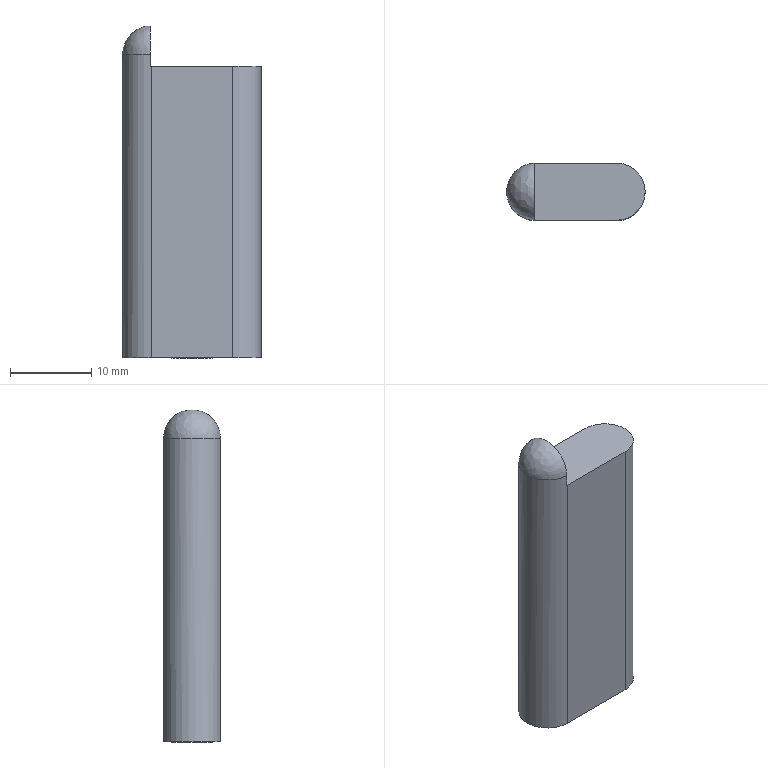Part | STEP file | LUOI GA TRON DUOI | 1 solid | 15 faces | box 17 x 7 x 40.799 mm | volume 3679 mm3 | cylinder 5 | plane 5 | cone 4 | spline 1 | commonest cylinder face diameters 7 x3 4.134 x2
STEP:
#1=CARTESIAN_POINT('',(0.,0.,0.));
#2=DIRECTION('',(0.,0.,1.));
#3=DIRECTION('',(1.,0.,0.));
#4=AXIS2_PLACEMENT_3D('',#1,#2,#3);
#5=CARTESIAN_POINT('',(-3.5,0.,0.));
#6=VERTEX_POINT('',#5);
#7=CARTESIAN_POINT('',(0.,3.5,0.));
#8=VERTEX_POINT('',#7);
#9=CARTESIAN_POINT('',(-3.5,3.5,0.));
#10=DIRECTION('',(0.,0.,1.));
#11=DIRECTION('',(1.,0.,0.));
#12=AXIS2_PLACEMENT_3D('',#9,#10,#11);
#13=CIRCLE('',#12,3.5);
#14=CARTESIAN_POINT('',(-3.5,3.5,0.));
#15=DIRECTION('',(0.,0.,1.));
#16=DIRECTION('',(1.,0.,0.));
#17=AXIS2_PLACEMENT_3D('',#14,#15,#16);
#18=CYLINDRICAL_SURFACE('',#17,3.5);
#19=CARTESIAN_POINT('',(0.,0.));
#20=DIRECTION('',(1.,0.));
#21=VECTOR('',#20,1.);
#22=LINE('',#19,#21);
#23=(GEOMETRIC_REPRESENTATION_CONTEXT(2)PARAMETRIC_REPRESENTATION_CONTEXT()REPRESENTATION_CONTEXT('',''));
#24=DEFINITIONAL_REPRESENTATION('',(#22),#23);
#25=PCURVE('',#18,#24);
#26=CARTESIAN_POINT('',(-8.5,3.5,0.));
#27=DIRECTION('',(0.,0.,1.));
#28=DIRECTION('',(1.,0.,0.));
#29=AXIS2_PLACEMENT_3D('',#26,#27,#28);
#30=PLANE('',#29);
#31=CARTESIAN_POINT('',(5.,0.));
#32=DIRECTION('',(1.,0.));
#33=AXIS2_PLACEMENT_2D('',#31,#32);
#34=CIRCLE('',#33,3.5);
#35=(GEOMETRIC_REPRESENTATION_CONTEXT(2)PARAMETRIC_REPRESENTATION_CONTEXT()REPRESENTATION_CONTEXT('',''));
#36=DEFINITIONAL_REPRESENTATION('',(#34),#35);
#37=PCURVE('',#30,#36);
#38=SURFACE_CURVE('',#13,(#25,#37),.PCURVE_S1.);
#39=EDGE_CURVE('',#6,#8,#38,.T.);
#40=ORIENTED_EDGE('',*,*,#39,.T.);
#41=CARTESIAN_POINT('',(0.,3.5,35.8));
#42=VERTEX_POINT('',#41);
#43=CARTESIAN_POINT('',(0.,3.5,0.));
#44=DIRECTION('',(0.,0.,1.));
#45=VECTOR('',#44,1.);
#46=LINE('',#43,#45);
#47=CARTESIAN_POINT('',(6.283,0.));
#48=DIRECTION('',(0.,1.));
#49=VECTOR('',#48,1.);
#50=LINE('',#47,#49);
#51=(GEOMETRIC_REPRESENTATION_CONTEXT(2)PARAMETRIC_REPRESENTATION_CONTEXT()REPRESENTATION_CONTEXT('',''));
#52=DEFINITIONAL_REPRESENTATION('',(#50),#51);
#53=PCURVE('',#18,#52);
#54=CARTESIAN_POINT('',(-3.5,3.5,0.));
#55=DIRECTION('',(0.,0.,1.));
#56=DIRECTION('',(1.,0.,0.));
#57=AXIS2_PLACEMENT_3D('',#54,#55,#56);
#58=CYLINDRICAL_SURFACE('',#57,3.5);
#59=CARTESIAN_POINT('',(0.,0.));
#60=DIRECTION('',(0.,1.));
#61=VECTOR('',#60,1.);
#62=LINE('',#59,#61);
#63=(GEOMETRIC_REPRESENTATION_CONTEXT(2)PARAMETRIC_REPRESENTATION_CONTEXT()REPRESENTATION_CONTEXT('',''));
#64=DEFINITIONAL_REPRESENTATION('',(#62),#63);
#65=PCURVE('',#58,#64);
#66=SURFACE_CURVE('',#46,(#53,#65),.PCURVE_S1.);
#67=EDGE_CURVE('',#8,#42,#66,.T.);
#68=ORIENTED_EDGE('',*,*,#67,.T.);
#69=CARTESIAN_POINT('',(-3.5,0.,35.8));
#70=VERTEX_POINT('',#69);
#71=CARTESIAN_POINT('',(-3.5,3.5,35.8));
#72=DIRECTION('',(0.,0.,-1.));
#73=DIRECTION('',(1.,0.,0.));
#74=AXIS2_PLACEMENT_3D('',#71,#72,#73);
#75=CIRCLE('',#74,3.5);
#76=CARTESIAN_POINT('',(6.283,35.8));
#77=DIRECTION('',(-1.,0.));
#78=VECTOR('',#77,1.);
#79=LINE('',#76,#78);
#80=(GEOMETRIC_REPRESENTATION_CONTEXT(2)PARAMETRIC_REPRESENTATION_CONTEXT()REPRESENTATION_CONTEXT('',''));
#81=DEFINITIONAL_REPRESENTATION('',(#79),#80);
#82=PCURVE('',#18,#81);
#83=CARTESIAN_POINT('',(-13.6,0.,35.8));
#84=DIRECTION('',(0.,0.,-1.));
#85=DIRECTION('',(-1.,0.,0.));
#86=AXIS2_PLACEMENT_3D('',#83,#84,#85);
#87=PLANE('',#86);
#88=CARTESIAN_POINT('',(-10.1,3.5));
#89=DIRECTION('',(-1.,0.));
#90=AXIS2_PLACEMENT_2D('',#88,#89);
#91=CIRCLE('',#90,3.5);
#92=(GEOMETRIC_REPRESENTATION_CONTEXT(2)PARAMETRIC_REPRESENTATION_CONTEXT()REPRESENTATION_CONTEXT('',''));
#93=DEFINITIONAL_REPRESENTATION('',(#91),#92);
#94=PCURVE('',#87,#93);
#95=SURFACE_CURVE('',#75,(#82,#94),.PCURVE_S1.);
#96=EDGE_CURVE('',#42,#70,#95,.T.);
#97=ORIENTED_EDGE('',*,*,#96,.T.);
#98=CARTESIAN_POINT('',(-3.5,0.,0.));
#99=DIRECTION('',(0.,0.,1.));
#100=VECTOR('',#99,1.);
#101=LINE('',#98,#100);
#102=CARTESIAN_POINT('',(4.712,0.));
#103=DIRECTION('',(0.,1.));
#104=VECTOR('',#103,1.);
#105=LINE('',#102,#104);
#106=(GEOMETRIC_REPRESENTATION_CONTEXT(2)PARAMETRIC_REPRESENTATION_CONTEXT()REPRESENTATION_CONTEXT('',''));
#107=DEFINITIONAL_REPRESENTATION('',(#105),#106);
#108=PCURVE('',#18,#107);
#109=CARTESIAN_POINT('',(0.,0.,0.));
#110=DIRECTION('',(0.,-1.,0.));
#111=DIRECTION('',(0.,0.,-1.));
#112=AXIS2_PLACEMENT_3D('',#109,#110,#111);
#113=PLANE('',#112);
#114=CARTESIAN_POINT('',(0.,-3.5));
#115=DIRECTION('',(-1.,0.));
#116=VECTOR('',#115,1.);
#117=LINE('',#114,#116);
#118=(GEOMETRIC_REPRESENTATION_CONTEXT(2)PARAMETRIC_REPRESENTATION_CONTEXT()REPRESENTATION_CONTEXT('',''));
#119=DEFINITIONAL_REPRESENTATION('',(#117),#118);
#120=PCURVE('',#113,#119);
#121=SURFACE_CURVE('',#101,(#108,#120),.PCURVE_S1.);
#122=EDGE_CURVE('',#6,#70,#121,.T.);
#123=ORIENTED_EDGE('',*,*,#122,.F.);
#124=EDGE_LOOP('',(#40,#68,#97,#123));
#125=FACE_BOUND('',#124,.T.);
#126=ADVANCED_FACE('',(#125),#18,.T.);
#127=CARTESIAN_POINT('',(-10.567,3.5,0.5));
#128=VERTEX_POINT('',#127);
#129=CARTESIAN_POINT('',(-11.067,3.5,0.));
#130=VERTEX_POINT('',#129);
#131=CARTESIAN_POINT('',(-11.067,3.5,0.));
#132=DIRECTION('',(-0.7071,0.,-0.7071));
#133=VECTOR('',#132,1.);
#134=LINE('',#131,#133);
#135=CARTESIAN_POINT('',(-8.5,3.5,0.));
#136=DIRECTION('',(0.,0.,-1.));
#137=DIRECTION('',(-1.,0.,0.));
#138=AXIS2_PLACEMENT_3D('',#135,#136,#137);
#139=CONICAL_SURFACE('',#138,2.567,0.7854);
#140=CARTESIAN_POINT('',(6.283,0.));
#141=DIRECTION('',(0.,1.));
#142=VECTOR('',#141,1.);
#143=LINE('',#140,#142);
#144=(GEOMETRIC_REPRESENTATION_CONTEXT(2)PARAMETRIC_REPRESENTATION_CONTEXT()REPRESENTATION_CONTEXT('',''));
#145=DEFINITIONAL_REPRESENTATION('',(#143),#144);
#146=PCURVE('',#139,#145);
#147=CARTESIAN_POINT('',(-8.5,3.5,0.));
#148=DIRECTION('',(0.,0.,-1.));
#149=DIRECTION('',(-1.,0.,0.));
#150=AXIS2_PLACEMENT_3D('',#147,#148,#149);
#151=CONICAL_SURFACE('',#150,2.567,0.7854);
#152=CARTESIAN_POINT('',(0.,0.));
#153=DIRECTION('',(0.,1.));
#154=VECTOR('',#153,1.);
#155=LINE('',#152,#154);
#156=(GEOMETRIC_REPRESENTATION_CONTEXT(2)PARAMETRIC_REPRESENTATION_CONTEXT()REPRESENTATION_CONTEXT('',''));
#157=DEFINITIONAL_REPRESENTATION('',(#155),#156);
#158=PCURVE('',#151,#157);
#159=SURFACE_CURVE('',#134,(#146,#158),.PCURVE_S1.);
#160=EDGE_CURVE('',#128,#130,#159,.T.);
#161=ORIENTED_EDGE('',*,*,#160,.T.);
#162=CARTESIAN_POINT('',(-5.933,3.5,0.));
#163=VERTEX_POINT('',#162);
#164=CARTESIAN_POINT('',(-8.5,3.5,0.));
#165=DIRECTION('',(0.,0.,-1.));
#166=DIRECTION('',(-1.,0.,0.));
#167=AXIS2_PLACEMENT_3D('',#164,#165,#166);
#168=CIRCLE('',#167,2.567);
#169=CARTESIAN_POINT('',(0.,0.));
#170=DIRECTION('',(1.,0.));
#171=VECTOR('',#170,1.);
#172=LINE('',#169,#171);
#173=(GEOMETRIC_REPRESENTATION_CONTEXT(2)PARAMETRIC_REPRESENTATION_CONTEXT()REPRESENTATION_CONTEXT('',''));
#174=DEFINITIONAL_REPRESENTATION('',(#172),#173);
#175=PCURVE('',#139,#174);
#176=CARTESIAN_POINT('',(-2.567,0.));
#177=CARTESIAN_POINT('',(-2.567,4.446));
#178=CARTESIAN_POINT('',(1.283,2.223));
#179=CARTESIAN_POINT('',(5.134,0.));
#180=CARTESIAN_POINT('',(1.283,-2.223));
#181=CARTESIAN_POINT('',(-2.567,-4.446));
#182=CARTESIAN_POINT('',(-2.567,0.));
#183=(BOUNDED_CURVE()B_SPLINE_CURVE(2,(#176,#177,#178,#179,#180,#181,#182),.UNSPECIFIED.,.T.,.F.)B_SPLINE_CURVE_WITH_KNOTS((1,2,2,2,2,1),(-2.094,0.,2.094,4.189,6.283,8.378),.UNSPECIFIED.)CURVE()GEOMETRIC_REPRESENTATION_ITEM()RATIONAL_B_SPLINE_CURVE((1.,0.5,1.,0.5,1.,0.5,1.))REPRESENTATION_ITEM(''));
#184=(GEOMETRIC_REPRESENTATION_CONTEXT(2)PARAMETRIC_REPRESENTATION_CONTEXT()REPRESENTATION_CONTEXT('',''));
#185=DEFINITIONAL_REPRESENTATION('',(#183),#184);
#186=PCURVE('',#30,#185);
#187=SURFACE_CURVE('',#168,(#175,#186),.PCURVE_S1.);
#188=EDGE_CURVE('',#163,#130,#187,.T.);
#189=ORIENTED_EDGE('',*,*,#188,.F.);
#190=CARTESIAN_POINT('',(-6.433,3.5,0.5));
#191=VERTEX_POINT('',#190);
#192=CARTESIAN_POINT('',(-5.933,3.5,0.));
#193=DIRECTION('',(0.7071,0.,-0.7071));
#194=VECTOR('',#193,1.);
#195=LINE('',#192,#194);
#196=CARTESIAN_POINT('',(3.142,0.));
#197=DIRECTION('',(0.,1.));
#198=VECTOR('',#197,1.);
#199=LINE('',#196,#198);
#200=(GEOMETRIC_REPRESENTATION_CONTEXT(2)PARAMETRIC_REPRESENTATION_CONTEXT()REPRESENTATION_CONTEXT('',''));
#201=DEFINITIONAL_REPRESENTATION('',(#199),#200);
#202=PCURVE('',#139,#201);
#203=CARTESIAN_POINT('',(3.142,0.));
#204=DIRECTION('',(0.,1.));
#205=VECTOR('',#204,1.);
#206=LINE('',#203,#205);
#207=(GEOMETRIC_REPRESENTATION_CONTEXT(2)PARAMETRIC_REPRESENTATION_CONTEXT()REPRESENTATION_CONTEXT('',''));
#208=DEFINITIONAL_REPRESENTATION('',(#206),#207);
#209=PCURVE('',#151,#208);
#210=SURFACE_CURVE('',#195,(#202,#209),.PCURVE_S1.);
#211=EDGE_CURVE('',#191,#163,#210,.T.);
#212=ORIENTED_EDGE('',*,*,#211,.F.);
#213=CARTESIAN_POINT('',(-8.5,3.5,0.5));
#214=DIRECTION('',(0.,0.,-1.));
#215=DIRECTION('',(1.,0.,0.));
#216=AXIS2_PLACEMENT_3D('',#213,#214,#215);
#217=CIRCLE('',#216,2.067);
#218=CARTESIAN_POINT('',(3.142,-0.5));
#219=DIRECTION('',(1.,0.));
#220=VECTOR('',#219,1.);
#221=LINE('',#218,#220);
#222=(GEOMETRIC_REPRESENTATION_CONTEXT(2)PARAMETRIC_REPRESENTATION_CONTEXT()REPRESENTATION_CONTEXT('',''));
#223=DEFINITIONAL_REPRESENTATION('',(#221),#222);
#224=PCURVE('',#139,#223);
#225=CARTESIAN_POINT('',(-8.5,3.5,10.));
#226=DIRECTION('',(0.,0.,-1.));
#227=DIRECTION('',(-1.,0.,0.));
#228=AXIS2_PLACEMENT_3D('',#225,#226,#227);
#229=CYLINDRICAL_SURFACE('',#228,2.067);
#230=CARTESIAN_POINT('',(3.142,9.5));
#231=DIRECTION('',(1.,0.));
#232=VECTOR('',#231,1.);
#233=LINE('',#230,#232);
#234=(GEOMETRIC_REPRESENTATION_CONTEXT(2)PARAMETRIC_REPRESENTATION_CONTEXT()REPRESENTATION_CONTEXT('',''));
#235=DEFINITIONAL_REPRESENTATION('',(#233),#234);
#236=PCURVE('',#229,#235);
#237=SURFACE_CURVE('',#217,(#224,#236),.PCURVE_S1.);
#238=EDGE_CURVE('',#191,#128,#237,.T.);
#239=ORIENTED_EDGE('',*,*,#238,.T.);
#240=EDGE_LOOP('',(#161,#189,#212,#239));
#241=FACE_BOUND('',#240,.F.);
#242=ADVANCED_FACE('',(#241),#139,.F.);
#243=CARTESIAN_POINT('',(-10.567,3.5,20.));
#244=VERTEX_POINT('',#243);
#245=CARTESIAN_POINT('',(-10.567,3.5,10.));
#246=DIRECTION('',(0.,0.,-1.));
#247=VECTOR('',#246,1.);
#248=LINE('',#245,#247);
#249=CARTESIAN_POINT('',(6.283,0.));
#250=DIRECTION('',(0.,1.));
#251=VECTOR('',#250,1.);
#252=LINE('',#249,#251);
#253=(GEOMETRIC_REPRESENTATION_CONTEXT(2)PARAMETRIC_REPRESENTATION_CONTEXT()REPRESENTATION_CONTEXT('',''));
#254=DEFINITIONAL_REPRESENTATION('',(#252),#253);
#255=PCURVE('',#229,#254);
#256=CARTESIAN_POINT('',(-8.5,3.5,10.));
#257=DIRECTION('',(0.,0.,-1.));
#258=DIRECTION('',(-1.,0.,0.));
#259=AXIS2_PLACEMENT_3D('',#256,#257,#258);
#260=CYLINDRICAL_SURFACE('',#259,2.067);
#261=CARTESIAN_POINT('',(0.,0.));
#262=DIRECTION('',(0.,1.));
#263=VECTOR('',#262,1.);
#264=LINE('',#261,#263);
#265=(GEOMETRIC_REPRESENTATION_CONTEXT(2)PARAMETRIC_REPRESENTATION_CONTEXT()REPRESENTATION_CONTEXT('',''));
#266=DEFINITIONAL_REPRESENTATION('',(#264),#265);
#267=PCURVE('',#260,#266);
#268=SURFACE_CURVE('',#248,(#255,#267),.PCURVE_S1.);
#269=EDGE_CURVE('',#244,#128,#268,.T.);
#270=ORIENTED_EDGE('',*,*,#269,.T.);
#271=ORIENTED_EDGE('',*,*,#238,.F.);
#272=CARTESIAN_POINT('',(-6.433,3.5,20.));
#273=VERTEX_POINT('',#272);
#274=CARTESIAN_POINT('',(-6.433,3.5,10.));
#275=DIRECTION('',(0.,0.,-1.));
#276=VECTOR('',#275,1.);
#277=LINE('',#274,#276);
#278=CARTESIAN_POINT('',(3.142,0.));
#279=DIRECTION('',(0.,1.));
#280=VECTOR('',#279,1.);
#281=LINE('',#278,#280);
#282=(GEOMETRIC_REPRESENTATION_CONTEXT(2)PARAMETRIC_REPRESENTATION_CONTEXT()REPRESENTATION_CONTEXT('',''));
#283=DEFINITIONAL_REPRESENTATION('',(#281),#282);
#284=PCURVE('',#229,#283);
#285=CARTESIAN_POINT('',(3.142,0.));
#286=DIRECTION('',(0.,1.));
#287=VECTOR('',#286,1.);
#288=LINE('',#285,#287);
#289=(GEOMETRIC_REPRESENTATION_CONTEXT(2)PARAMETRIC_REPRESENTATION_CONTEXT()REPRESENTATION_CONTEXT('',''));
#290=DEFINITIONAL_REPRESENTATION('',(#288),#289);
#291=PCURVE('',#260,#290);
#292=SURFACE_CURVE('',#277,(#284,#291),.PCURVE_S1.);
#293=EDGE_CURVE('',#273,#191,#292,.T.);
#294=ORIENTED_EDGE('',*,*,#293,.F.);
#295=CARTESIAN_POINT('',(-8.5,3.5,20.));
#296=DIRECTION('',(0.,0.,-1.));
#297=DIRECTION('',(-1.,0.,0.));
#298=AXIS2_PLACEMENT_3D('',#295,#296,#297);
#299=CIRCLE('',#298,2.067);
#300=CARTESIAN_POINT('',(0.,-10.));
#301=DIRECTION('',(1.,0.));
#302=VECTOR('',#301,1.);
#303=LINE('',#300,#302);
#304=(GEOMETRIC_REPRESENTATION_CONTEXT(2)PARAMETRIC_REPRESENTATION_CONTEXT()REPRESENTATION_CONTEXT('',''));
#305=DEFINITIONAL_REPRESENTATION('',(#303),#304);
#306=PCURVE('',#229,#305);
#307=CARTESIAN_POINT('',(-8.5,3.5,20.));
#308=DIRECTION('',(0.,0.,-1.));
#309=DIRECTION('',(-1.,0.,0.));
#310=AXIS2_PLACEMENT_3D('',#307,#308,#309);
#311=CONICAL_SURFACE('',#310,2.067,1.03);
#312=CARTESIAN_POINT('',(0.,0.));
#313=DIRECTION('',(1.,0.));
#314=VECTOR('',#313,1.);
#315=LINE('',#312,#314);
#316=(GEOMETRIC_REPRESENTATION_CONTEXT(2)PARAMETRIC_REPRESENTATION_CONTEXT()REPRESENTATION_CONTEXT('',''));
#317=DEFINITIONAL_REPRESENTATION('',(#315),#316);
#318=PCURVE('',#311,#317);
#319=SURFACE_CURVE('',#299,(#306,#318),.PCURVE_S1.);
#320=EDGE_CURVE('',#273,#244,#319,.T.);
#321=ORIENTED_EDGE('',*,*,#320,.T.);
#322=EDGE_LOOP('',(#270,#271,#294,#321));
#323=FACE_BOUND('',#322,.F.);
#324=ADVANCED_FACE('',(#323),#229,.F.);
#325=ORIENTED_EDGE('',*,*,#320,.F.);
#326=CARTESIAN_POINT('',(-8.5,3.5,21.242));
#327=VERTEX_POINT('',#326);
#328=CARTESIAN_POINT('',(-6.433,3.5,20.));
#329=DIRECTION('',(0.8572,0.,-0.515));
#330=VECTOR('',#329,1.);
#331=LINE('',#328,#330);
#332=CARTESIAN_POINT('',(3.142,0.));
#333=DIRECTION('',(0.,1.));
#334=VECTOR('',#333,1.);
#335=LINE('',#332,#334);
#336=(GEOMETRIC_REPRESENTATION_CONTEXT(2)PARAMETRIC_REPRESENTATION_CONTEXT()REPRESENTATION_CONTEXT('',''));
#337=DEFINITIONAL_REPRESENTATION('',(#335),#336);
#338=PCURVE('',#311,#337);
#339=CARTESIAN_POINT('',(-8.5,3.5,20.));
#340=DIRECTION('',(0.,0.,-1.));
#341=DIRECTION('',(-1.,0.,0.));
#342=AXIS2_PLACEMENT_3D('',#339,#340,#341);
#343=CONICAL_SURFACE('',#342,2.067,1.03);
#344=CARTESIAN_POINT('',(3.142,0.));
#345=DIRECTION('',(0.,1.));
#346=VECTOR('',#345,1.);
#347=LINE('',#344,#346);
#348=(GEOMETRIC_REPRESENTATION_CONTEXT(2)PARAMETRIC_REPRESENTATION_CONTEXT()REPRESENTATION_CONTEXT('',''));
#349=DEFINITIONAL_REPRESENTATION('',(#347),#348);
#350=PCURVE('',#343,#349);
#351=SURFACE_CURVE('',#331,(#338,#350),.PCURVE_S1.);
#352=EDGE_CURVE('',#327,#273,#351,.T.);
#353=ORIENTED_EDGE('',*,*,#352,.F.);
#354=CARTESIAN_POINT('',(-10.567,3.5,20.));
#355=DIRECTION('',(-0.8572,0.,-0.515));
#356=VECTOR('',#355,1.);
#357=LINE('',#354,#356);
#358=CARTESIAN_POINT('',(6.283,0.));
#359=DIRECTION('',(0.,1.));
#360=VECTOR('',#359,1.);
#361=LINE('',#358,#360);
#362=(GEOMETRIC_REPRESENTATION_CONTEXT(2)PARAMETRIC_REPRESENTATION_CONTEXT()REPRESENTATION_CONTEXT('',''));
#363=DEFINITIONAL_REPRESENTATION('',(#361),#362);
#364=PCURVE('',#311,#363);
#365=CARTESIAN_POINT('',(0.,0.));
#366=DIRECTION('',(0.,1.));
#367=VECTOR('',#366,1.);
#368=LINE('',#365,#367);
#369=(GEOMETRIC_REPRESENTATION_CONTEXT(2)PARAMETRIC_REPRESENTATION_CONTEXT()REPRESENTATION_CONTEXT('',''));
#370=DEFINITIONAL_REPRESENTATION('',(#368),#369);
#371=PCURVE('',#343,#370);
#372=SURFACE_CURVE('',#357,(#364,#371),.PCURVE_S1.);
#373=EDGE_CURVE('',#327,#244,#372,.T.);
#374=ORIENTED_EDGE('',*,*,#373,.T.);
#375=EDGE_LOOP('',(#325,#353,#374));
#376=FACE_BOUND('',#375,.F.);
#377=ADVANCED_FACE('',(#376),#311,.F.);
#378=CARTESIAN_POINT('',(-13.5,0.,35.8));
#379=VERTEX_POINT('',#378);
#380=CARTESIAN_POINT('',(-13.6,0.001429,35.8));
#381=VERTEX_POINT('',#380);
#382=CARTESIAN_POINT('',(-13.5,3.5,35.8));
#383=DIRECTION('',(0.,0.,-1.));
#384=DIRECTION('',(1.,0.,0.));
#385=AXIS2_PLACEMENT_3D('',#382,#383,#384);
#386=CIRCLE('',#385,3.5);
#387=CARTESIAN_POINT('',(-13.5,3.5,0.));
#388=DIRECTION('',(0.,0.,1.));
#389=DIRECTION('',(1.,0.,0.));
#390=AXIS2_PLACEMENT_3D('',#387,#388,#389);
#391=CYLINDRICAL_SURFACE('',#390,3.5);
#392=CARTESIAN_POINT('',(6.283,35.8));
#393=DIRECTION('',(-1.,0.));
#394=VECTOR('',#393,1.);
#395=LINE('',#392,#394);
#396=(GEOMETRIC_REPRESENTATION_CONTEXT(2)PARAMETRIC_REPRESENTATION_CONTEXT()REPRESENTATION_CONTEXT('',''));
#397=DEFINITIONAL_REPRESENTATION('',(#395),#396);
#398=PCURVE('',#391,#397);
#399=CARTESIAN_POINT('',(-0.1,3.5));
#400=DIRECTION('',(-1.,0.));
#401=AXIS2_PLACEMENT_2D('',#399,#400);
#402=CIRCLE('',#401,3.5);
#403=(GEOMETRIC_REPRESENTATION_CONTEXT(2)PARAMETRIC_REPRESENTATION_CONTEXT()REPRESENTATION_CONTEXT('',''));
#404=DEFINITIONAL_REPRESENTATION('',(#402),#403);
#405=PCURVE('',#87,#404);
#406=SURFACE_CURVE('',#386,(#398,#405),.PCURVE_S1.);
#407=EDGE_CURVE('',#379,#381,#406,.T.);
#408=ORIENTED_EDGE('',*,*,#407,.T.);
#409=CARTESIAN_POINT('',(-13.6,0.001429,37.3));
#410=VERTEX_POINT('',#409);
#411=CARTESIAN_POINT('',(-13.6,0.001429,40.8));
#412=DIRECTION('',(0.,0.,1.));
#413=VECTOR('',#412,1.);
#414=LINE('',#411,#413);
#415=CARTESIAN_POINT('',(4.684,40.8));
#416=DIRECTION('',(0.,1.));
#417=VECTOR('',#416,1.);
#418=LINE('',#415,#417);
#419=(GEOMETRIC_REPRESENTATION_CONTEXT(2)PARAMETRIC_REPRESENTATION_CONTEXT()REPRESENTATION_CONTEXT('',''));
#420=DEFINITIONAL_REPRESENTATION('',(#418),#419);
#421=PCURVE('',#391,#420);
#422=CARTESIAN_POINT('',(-13.6,0.,40.8));
#423=DIRECTION('',(-1.,0.,0.));
#424=DIRECTION('',(0.,0.,1.));
#425=AXIS2_PLACEMENT_3D('',#422,#423,#424);
#426=PLANE('',#425);
#427=CARTESIAN_POINT('',(0.,0.001429));
#428=DIRECTION('',(1.,0.));
#429=VECTOR('',#428,1.);
#430=LINE('',#427,#429);
#431=(GEOMETRIC_REPRESENTATION_CONTEXT(2)PARAMETRIC_REPRESENTATION_CONTEXT()REPRESENTATION_CONTEXT('',''));
#432=DEFINITIONAL_REPRESENTATION('',(#430),#431);
#433=PCURVE('',#426,#432);
#434=SURFACE_CURVE('',#414,(#421,#433),.PCURVE_S1.);
#435=EDGE_CURVE('',#381,#410,#434,.T.);
#436=ORIENTED_EDGE('',*,*,#435,.T.);
#437=CARTESIAN_POINT('',(-17.,3.5,37.3));
#438=VERTEX_POINT('',#437);
#439=CARTESIAN_POINT('',(-13.5,3.5,37.3));
#440=DIRECTION('',(0.,0.,-1.));
#441=DIRECTION('',(1.,0.,0.));
#442=AXIS2_PLACEMENT_3D('',#439,#440,#441);
#443=CIRCLE('',#442,3.5);
#444=CARTESIAN_POINT('',(6.283,37.3));
#445=DIRECTION('',(-1.,0.));
#446=VECTOR('',#445,1.);
#447=LINE('',#444,#446);
#448=(GEOMETRIC_REPRESENTATION_CONTEXT(2)PARAMETRIC_REPRESENTATION_CONTEXT()REPRESENTATION_CONTEXT('',''));
#449=DEFINITIONAL_REPRESENTATION('',(#447),#448);
#450=PCURVE('',#391,#449);
#451=CARTESIAN_POINT('',(-13.6,6.999,37.3));
#452=CARTESIAN_POINT('',(-13.6,6.999,44.297));
#453=CARTESIAN_POINT('',(-13.6,0.001429,44.297));
#454=CARTESIAN_POINT('',(-13.6,0.001429,37.3));
#455=CARTESIAN_POINT('',(-15.603,6.941,37.3));
#456=CARTESIAN_POINT('',(-15.603,6.941,44.183));
#457=CARTESIAN_POINT('',(-15.603,0.05869,44.183));
#458=CARTESIAN_POINT('',(-15.603,0.05869,37.3));
#459=CARTESIAN_POINT('',(-17.,5.504,37.3));
#460=CARTESIAN_POINT('',(-17.,5.504,41.308));
#461=CARTESIAN_POINT('',(-17.,1.496,41.308));
#462=CARTESIAN_POINT('',(-17.,1.496,37.3));
#463=CARTESIAN_POINT('',(-17.,3.5,37.3));
#464=CARTESIAN_POINT('',(-17.,3.5,37.3));
#465=CARTESIAN_POINT('',(-17.,3.5,37.3));
#466=CARTESIAN_POINT('',(-17.,3.5,37.3));
#467=(BOUNDED_SURFACE()B_SPLINE_SURFACE(3,3,((#451,#452,#453,#454),(#455,#456,#457,#458),(#459,#460,#461,#462),(#463,#464,#465,#466)),.UNSPECIFIED.,.F.,.F.,.F.)B_SPLINE_SURFACE_WITH_KNOTS((4,4),(4,4),(0.,1.),(0.,1.),.PIECEWISE_BEZIER_KNOTS.)GEOMETRIC_REPRESENTATION_ITEM()RATIONAL_B_SPLINE_SURFACE(((1.,0.3333,0.3333,1.),(0.8114,0.2705,0.2705,0.8114),(0.8114,0.2705,0.2705,0.8114),(1.,0.3333,0.3333,1.)))REPRESENTATION_ITEM('')SURFACE());
#468=CARTESIAN_POINT('',(0.,1.));
#469=CARTESIAN_POINT('',(0.01676,1.));
#470=CARTESIAN_POINT('',(0.04982,1.));
#471=CARTESIAN_POINT('',(0.09814,1.));
#472=CARTESIAN_POINT('',(0.1454,1.));
#473=CARTESIAN_POINT('',(0.1917,1.));
#474=CARTESIAN_POINT('',(0.2371,1.));
#475=CARTESIAN_POINT('',(0.282,1.));
#476=CARTESIAN_POINT('',(0.3262,1.));
#477=CARTESIAN_POINT('',(0.37,1.));
#478=CARTESIAN_POINT('',(0.4135,1.));
#479=CARTESIAN_POINT('',(0.4568,1.));
#480=CARTESIAN_POINT('',(0.5,1.));
#481=CARTESIAN_POINT('',(0.5432,1.));
#482=CARTESIAN_POINT('',(0.5865,1.));
#483=CARTESIAN_POINT('',(0.63,1.));
#484=CARTESIAN_POINT('',(0.6738,1.));
#485=CARTESIAN_POINT('',(0.718,1.));
#486=CARTESIAN_POINT('',(0.7629,1.));
#487=CARTESIAN_POINT('',(0.8083,1.));
#488=CARTESIAN_POINT('',(0.8546,1.));
#489=CARTESIAN_POINT('',(0.9019,1.));
#490=CARTESIAN_POINT('',(0.9502,1.));
#491=CARTESIAN_POINT('',(0.9832,1.));
#492=CARTESIAN_POINT('',(1.,1.));
#493=B_SPLINE_CURVE_WITH_KNOTS('',3,(#468,#469,#470,#471,#472,#473,#474,#475,#476,#477,#478,#479,#480,#481,#482,#483,#484,#485,#486,#487,#488,#489,#490,#491,#492),.UNSPECIFIED.,.F.,.F.,(4,1,1,1,1,1,1,1,1,1,1,1,1,1,1,1,1,1,1,1,1,1,4),(1.599,1.669,1.74,1.81,1.88,1.95,2.02,2.09,2.16,2.23,2.3,2.37,2.441,2.511,2.581,2.651,2.721,2.791,2.861,2.931,3.001,3.071,3.142),.QUASI_UNIFORM_KNOTS.);
#494=(GEOMETRIC_REPRESENTATION_CONTEXT(2)PARAMETRIC_REPRESENTATION_CONTEXT()REPRESENTATION_CONTEXT('',''));
#495=DEFINITIONAL_REPRESENTATION('',(#493),#494);
#496=PCURVE('',#467,#495);
#497=SURFACE_CURVE('',#443,(#450,#496),.PCURVE_S1.);
#498=EDGE_CURVE('',#410,#438,#497,.T.);
#499=ORIENTED_EDGE('',*,*,#498,.T.);
#500=CARTESIAN_POINT('',(-13.6,6.999,37.3));
#501=VERTEX_POINT('',#500);
#502=CARTESIAN_POINT('',(-13.5,3.5,37.3));
#503=DIRECTION('',(0.,0.,-1.));
#504=DIRECTION('',(1.,0.,0.));
#505=AXIS2_PLACEMENT_3D('',#502,#503,#504);
#506=CIRCLE('',#505,3.5);
#507=CARTESIAN_POINT('',(6.283,37.3));
#508=DIRECTION('',(-1.,0.));
#509=VECTOR('',#508,1.);
#510=LINE('',#507,#509);
#511=(GEOMETRIC_REPRESENTATION_CONTEXT(2)PARAMETRIC_REPRESENTATION_CONTEXT()REPRESENTATION_CONTEXT('',''));
#512=DEFINITIONAL_REPRESENTATION('',(#510),#511);
#513=PCURVE('',#391,#512);
#514=CARTESIAN_POINT('',(1.,0.));
#515=CARTESIAN_POINT('',(0.9832,0.));
#516=CARTESIAN_POINT('',(0.9502,0.));
#517=CARTESIAN_POINT('',(0.9019,0.));
#518=CARTESIAN_POINT('',(0.8546,0.));
#519=CARTESIAN_POINT('',(0.8083,0.));
#520=CARTESIAN_POINT('',(0.7629,0.));
#521=CARTESIAN_POINT('',(0.718,0.));
#522=CARTESIAN_POINT('',(0.6738,0.));
#523=CARTESIAN_POINT('',(0.63,0.));
#524=CARTESIAN_POINT('',(0.5865,0.));
#525=CARTESIAN_POINT('',(0.5432,0.));
#526=CARTESIAN_POINT('',(0.5,0.));
#527=CARTESIAN_POINT('',(0.4568,0.));
#528=CARTESIAN_POINT('',(0.4135,0.));
#529=CARTESIAN_POINT('',(0.37,0.));
#530=CARTESIAN_POINT('',(0.3262,0.));
#531=CARTESIAN_POINT('',(0.282,0.));
#532=CARTESIAN_POINT('',(0.2371,0.));
#533=CARTESIAN_POINT('',(0.1917,0.));
#534=CARTESIAN_POINT('',(0.1454,0.));
#535=CARTESIAN_POINT('',(0.09814,0.));
#536=CARTESIAN_POINT('',(0.04982,0.));
#537=CARTESIAN_POINT('',(0.01676,0.));
#538=CARTESIAN_POINT('',(0.,0.));
#539=B_SPLINE_CURVE_WITH_KNOTS('',3,(#514,#515,#516,#517,#518,#519,#520,#521,#522,#523,#524,#525,#526,#527,#528,#529,#530,#531,#532,#533,#534,#535,#536,#537,#538),.UNSPECIFIED.,.F.,.F.,(4,1,1,1,1,1,1,1,1,1,1,1,1,1,1,1,1,1,1,1,1,1,4),(3.142,3.212,3.282,3.352,3.422,3.492,3.562,3.632,3.702,3.773,3.843,3.913,3.983,4.053,4.123,4.193,4.263,4.333,4.403,4.474,4.544,4.614,4.684),.QUASI_UNIFORM_KNOTS.);
#540=(GEOMETRIC_REPRESENTATION_CONTEXT(2)PARAMETRIC_REPRESENTATION_CONTEXT()REPRESENTATION_CONTEXT('',''));
#541=DEFINITIONAL_REPRESENTATION('',(#539),#540);
#542=PCURVE('',#467,#541);
#543=SURFACE_CURVE('',#506,(#513,#542),.PCURVE_S1.);
#544=EDGE_CURVE('',#438,#501,#543,.T.);
#545=ORIENTED_EDGE('',*,*,#544,.T.);
#546=CARTESIAN_POINT('',(-13.6,6.999,35.8));
#547=VERTEX_POINT('',#546);
#548=CARTESIAN_POINT('',(-13.6,6.999,40.8));
#549=DIRECTION('',(0.,0.,-1.));
#550=VECTOR('',#549,1.);
#551=LINE('',#548,#550);
#552=CARTESIAN_POINT('',(1.599,40.8));
#553=DIRECTION('',(0.,-1.));
#554=VECTOR('',#553,1.);
#555=LINE('',#552,#554);
#556=(GEOMETRIC_REPRESENTATION_CONTEXT(2)PARAMETRIC_REPRESENTATION_CONTEXT()REPRESENTATION_CONTEXT('',''));
#557=DEFINITIONAL_REPRESENTATION('',(#555),#556);
#558=PCURVE('',#391,#557);
#559=CARTESIAN_POINT('',(0.,6.999));
#560=DIRECTION('',(-1.,0.));
#561=VECTOR('',#560,1.);
#562=LINE('',#559,#561);
#563=(GEOMETRIC_REPRESENTATION_CONTEXT(2)PARAMETRIC_REPRESENTATION_CONTEXT()REPRESENTATION_CONTEXT('',''));
#564=DEFINITIONAL_REPRESENTATION('',(#562),#563);
#565=PCURVE('',#426,#564);
#566=SURFACE_CURVE('',#551,(#558,#565),.PCURVE_S1.);
#567=EDGE_CURVE('',#501,#547,#566,.T.);
#568=ORIENTED_EDGE('',*,*,#567,.T.);
#569=CARTESIAN_POINT('',(-13.5,7.,35.8));
#570=VERTEX_POINT('',#569);
#571=CARTESIAN_POINT('',(-13.5,3.5,35.8));
#572=DIRECTION('',(0.,0.,-1.));
#573=DIRECTION('',(1.,0.,0.));
#574=AXIS2_PLACEMENT_3D('',#571,#572,#573);
#575=CIRCLE('',#574,3.5);
#576=CARTESIAN_POINT('',(6.283,35.8));
#577=DIRECTION('',(-1.,0.));
#578=VECTOR('',#577,1.);
#579=LINE('',#576,#578);
#580=(GEOMETRIC_REPRESENTATION_CONTEXT(2)PARAMETRIC_REPRESENTATION_CONTEXT()REPRESENTATION_CONTEXT('',''));
#581=DEFINITIONAL_REPRESENTATION('',(#579),#580);
#582=PCURVE('',#391,#581);
#583=CARTESIAN_POINT('',(-0.1,3.5));
#584=DIRECTION('',(-1.,0.));
#585=AXIS2_PLACEMENT_2D('',#583,#584);
#586=CIRCLE('',#585,3.5);
#587=(GEOMETRIC_REPRESENTATION_CONTEXT(2)PARAMETRIC_REPRESENTATION_CONTEXT()REPRESENTATION_CONTEXT('',''));
#588=DEFINITIONAL_REPRESENTATION('',(#586),#587);
#589=PCURVE('',#87,#588);
#590=SURFACE_CURVE('',#575,(#582,#589),.PCURVE_S1.);
#591=EDGE_CURVE('',#547,#570,#590,.T.);
#592=ORIENTED_EDGE('',*,*,#591,.T.);
#593=CARTESIAN_POINT('',(-13.5,7.,0.));
#594=VERTEX_POINT('',#593);
#595=CARTESIAN_POINT('',(-13.5,7.,0.));
#596=DIRECTION('',(0.,0.,-1.));
#597=VECTOR('',#596,1.);
#598=LINE('',#595,#597);
#599=CARTESIAN_POINT('',(1.571,0.));
#600=DIRECTION('',(0.,-1.));
#601=VECTOR('',#600,1.);
#602=LINE('',#599,#601);
#603=(GEOMETRIC_REPRESENTATION_CONTEXT(2)PARAMETRIC_REPRESENTATION_CONTEXT()REPRESENTATION_CONTEXT('',''));
#604=DEFINITIONAL_REPRESENTATION('',(#602),#603);
#605=PCURVE('',#391,#604);
#606=CARTESIAN_POINT('',(-17.,7.,0.));
#607=DIRECTION('',(0.,1.,0.));
#608=DIRECTION('',(0.,0.,1.));
#609=AXIS2_PLACEMENT_3D('',#606,#607,#608);
#610=PLANE('',#609);
#611=CARTESIAN_POINT('',(0.,3.5));
#612=DIRECTION('',(-1.,0.));
#613=VECTOR('',#612,1.);
#614=LINE('',#611,#613);
#615=(GEOMETRIC_REPRESENTATION_CONTEXT(2)PARAMETRIC_REPRESENTATION_CONTEXT()REPRESENTATION_CONTEXT('',''));
#616=DEFINITIONAL_REPRESENTATION('',(#614),#615);
#617=PCURVE('',#610,#616);
#618=SURFACE_CURVE('',#598,(#605,#617),.PCURVE_S1.);
#619=EDGE_CURVE('',#570,#594,#618,.T.);
#620=ORIENTED_EDGE('',*,*,#619,.T.);
#621=CARTESIAN_POINT('',(-13.5,0.,0.));
#622=VERTEX_POINT('',#621);
#623=CARTESIAN_POINT('',(-13.5,3.5,0.));
#624=DIRECTION('',(0.,0.,1.));
#625=DIRECTION('',(1.,0.,0.));
#626=AXIS2_PLACEMENT_3D('',#623,#624,#625);
#627=CIRCLE('',#626,3.5);
#628=CARTESIAN_POINT('',(0.,0.));
#629=DIRECTION('',(1.,0.));
#630=VECTOR('',#629,1.);
#631=LINE('',#628,#630);
#632=(GEOMETRIC_REPRESENTATION_CONTEXT(2)PARAMETRIC_REPRESENTATION_CONTEXT()REPRESENTATION_CONTEXT('',''));
#633=DEFINITIONAL_REPRESENTATION('',(#631),#632);
#634=PCURVE('',#391,#633);
#635=CARTESIAN_POINT('',(-5.,0.));
#636=DIRECTION('',(1.,0.));
#637=AXIS2_PLACEMENT_2D('',#635,#636);
#638=CIRCLE('',#637,3.5);
#639=(GEOMETRIC_REPRESENTATION_CONTEXT(2)PARAMETRIC_REPRESENTATION_CONTEXT()REPRESENTATION_CONTEXT('',''));
#640=DEFINITIONAL_REPRESENTATION('',(#638),#639);
#641=PCURVE('',#30,#640);
#642=SURFACE_CURVE('',#627,(#634,#641),.PCURVE_S1.);
#643=EDGE_CURVE('',#594,#622,#642,.T.);
#644=ORIENTED_EDGE('',*,*,#643,.T.);
#645=CARTESIAN_POINT('',(-13.5,0.,0.));
#646=DIRECTION('',(0.,0.,1.));
#647=VECTOR('',#646,1.);
#648=LINE('',#645,#647);
#649=CARTESIAN_POINT('',(4.712,0.));
#650=DIRECTION('',(0.,1.));
#651=VECTOR('',#650,1.);
#652=LINE('',#649,#651);
#653=(GEOMETRIC_REPRESENTATION_CONTEXT(2)PARAMETRIC_REPRESENTATION_CONTEXT()REPRESENTATION_CONTEXT('',''));
#654=DEFINITIONAL_REPRESENTATION('',(#652),#653);
#655=PCURVE('',#391,#654);
#656=CARTESIAN_POINT('',(0.,-13.5));
#657=DIRECTION('',(-1.,0.));
#658=VECTOR('',#657,1.);
#659=LINE('',#656,#658);
#660=(GEOMETRIC_REPRESENTATION_CONTEXT(2)PARAMETRIC_REPRESENTATION_CONTEXT()REPRESENTATION_CONTEXT('',''));
#661=DEFINITIONAL_REPRESENTATION('',(#659),#660);
#662=PCURVE('',#113,#661);
#663=SURFACE_CURVE('',#648,(#655,#662),.PCURVE_S1.);
#664=EDGE_CURVE('',#622,#379,#663,.T.);
#665=ORIENTED_EDGE('',*,*,#664,.T.);
#666=EDGE_LOOP('',(#408,#436,#499,#545,#568,#592,#620,#644,#665));
#667=FACE_BOUND('',#666,.T.);
#668=ADVANCED_FACE('',(#667),#391,.T.);
#669=CARTESIAN_POINT('',(0.,0.,0.));
#670=DIRECTION('',(1.,0.,0.));
#671=VECTOR('',#670,1.);
#672=LINE('',#669,#671);
#673=CARTESIAN_POINT('',(0.,0.));
#674=DIRECTION('',(0.,1.));
#675=VECTOR('',#674,1.);
#676=LINE('',#673,#675);
#677=(GEOMETRIC_REPRESENTATION_CONTEXT(2)PARAMETRIC_REPRESENTATION_CONTEXT()REPRESENTATION_CONTEXT('',''));
#678=DEFINITIONAL_REPRESENTATION('',(#676),#677);
#679=PCURVE('',#113,#678);
#680=CARTESIAN_POINT('',(8.5,-3.5));
#681=DIRECTION('',(1.,0.));
#682=VECTOR('',#681,1.);
#683=LINE('',#680,#682);
#684=(GEOMETRIC_REPRESENTATION_CONTEXT(2)PARAMETRIC_REPRESENTATION_CONTEXT()REPRESENTATION_CONTEXT('',''));
#685=DEFINITIONAL_REPRESENTATION('',(#683),#684);
#686=PCURVE('',#30,#685);
#687=SURFACE_CURVE('',#672,(#679,#686),.PCURVE_S1.);
#688=EDGE_CURVE('',#622,#6,#687,.T.);
#689=ORIENTED_EDGE('',*,*,#688,.T.);
#690=ORIENTED_EDGE('',*,*,#122,.T.);
#691=CARTESIAN_POINT('',(0.,0.,35.8));
#692=DIRECTION('',(-1.,0.,0.));
#693=VECTOR('',#692,1.);
#694=LINE('',#691,#693);
#695=CARTESIAN_POINT('',(-35.8,0.));
#696=DIRECTION('',(0.,-1.));
#697=VECTOR('',#696,1.);
#698=LINE('',#695,#697);
#699=(GEOMETRIC_REPRESENTATION_CONTEXT(2)PARAMETRIC_REPRESENTATION_CONTEXT()REPRESENTATION_CONTEXT('',''));
#700=DEFINITIONAL_REPRESENTATION('',(#698),#699);
#701=PCURVE('',#113,#700);
#702=CARTESIAN_POINT('',(-13.6,0.));
#703=DIRECTION('',(1.,0.));
#704=VECTOR('',#703,1.);
#705=LINE('',#702,#704);
#706=(GEOMETRIC_REPRESENTATION_CONTEXT(2)PARAMETRIC_REPRESENTATION_CONTEXT()REPRESENTATION_CONTEXT('',''));
#707=DEFINITIONAL_REPRESENTATION('',(#705),#706);
#708=PCURVE('',#87,#707);
#709=SURFACE_CURVE('',#694,(#701,#708),.PCURVE_S1.);
#710=EDGE_CURVE('',#70,#379,#709,.T.);
#711=ORIENTED_EDGE('',*,*,#710,.T.);
#712=ORIENTED_EDGE('',*,*,#664,.F.);
#713=EDGE_LOOP('',(#689,#690,#711,#712));
#714=FACE_BOUND('',#713,.T.);
#715=ADVANCED_FACE('',(#714),#113,.T.);
#716=CARTESIAN_POINT('',(-8.5,3.5,0.));
#717=DIRECTION('',(0.,0.,-1.));
#718=DIRECTION('',(-1.,0.,0.));
#719=AXIS2_PLACEMENT_3D('',#716,#717,#718);
#720=CIRCLE('',#719,2.567);
#721=CARTESIAN_POINT('',(-2.567,0.));
#722=CARTESIAN_POINT('',(-2.567,4.446));
#723=CARTESIAN_POINT('',(1.283,2.223));
#724=CARTESIAN_POINT('',(5.134,0.));
#725=CARTESIAN_POINT('',(1.283,-2.223));
#726=CARTESIAN_POINT('',(-2.567,-4.446));
#727=CARTESIAN_POINT('',(-2.567,0.));
#728=(BOUNDED_CURVE()B_SPLINE_CURVE(2,(#721,#722,#723,#724,#725,#726,#727),.UNSPECIFIED.,.T.,.F.)B_SPLINE_CURVE_WITH_KNOTS((1,2,2,2,2,1),(-2.094,0.,2.094,4.189,6.283,8.378),.UNSPECIFIED.)CURVE()GEOMETRIC_REPRESENTATION_ITEM()RATIONAL_B_SPLINE_CURVE((1.,0.5,1.,0.5,1.,0.5,1.))REPRESENTATION_ITEM(''));
#729=(GEOMETRIC_REPRESENTATION_CONTEXT(2)PARAMETRIC_REPRESENTATION_CONTEXT()REPRESENTATION_CONTEXT('',''));
#730=DEFINITIONAL_REPRESENTATION('',(#728),#729);
#731=PCURVE('',#30,#730);
#732=CARTESIAN_POINT('',(0.,0.));
#733=DIRECTION('',(1.,0.));
#734=VECTOR('',#733,1.);
#735=LINE('',#732,#734);
#736=(GEOMETRIC_REPRESENTATION_CONTEXT(2)PARAMETRIC_REPRESENTATION_CONTEXT()REPRESENTATION_CONTEXT('',''));
#737=DEFINITIONAL_REPRESENTATION('',(#735),#736);
#738=PCURVE('',#151,#737);
#739=SURFACE_CURVE('',#720,(#731,#738),.PCURVE_S1.);
#740=EDGE_CURVE('',#130,#163,#739,.T.);
#741=ORIENTED_EDGE('',*,*,#740,.F.);
#742=ORIENTED_EDGE('',*,*,#188,.F.);
#743=EDGE_LOOP('',(#741,#742));
#744=FACE_BOUND('',#743,.T.);
#745=CARTESIAN_POINT('',(-3.5,7.,0.));
#746=VERTEX_POINT('',#745);
#747=CARTESIAN_POINT('',(-8.5,7.,0.));
#748=DIRECTION('',(-1.,0.,0.));
#749=VECTOR('',#748,1.);
#750=LINE('',#747,#749);
#751=CARTESIAN_POINT('',(0.,3.5));
#752=DIRECTION('',(-1.,0.));
#753=VECTOR('',#752,1.);
#754=LINE('',#751,#753);
#755=(GEOMETRIC_REPRESENTATION_CONTEXT(2)PARAMETRIC_REPRESENTATION_CONTEXT()REPRESENTATION_CONTEXT('',''));
#756=DEFINITIONAL_REPRESENTATION('',(#754),#755);
#757=PCURVE('',#30,#756);
#758=CARTESIAN_POINT('',(0.,8.5));
#759=DIRECTION('',(0.,-1.));
#760=VECTOR('',#759,1.);
#761=LINE('',#758,#760);
#762=(GEOMETRIC_REPRESENTATION_CONTEXT(2)PARAMETRIC_REPRESENTATION_CONTEXT()REPRESENTATION_CONTEXT('',''));
#763=DEFINITIONAL_REPRESENTATION('',(#761),#762);
#764=PCURVE('',#610,#763);
#765=SURFACE_CURVE('',#750,(#757,#764),.PCURVE_S1.);
#766=EDGE_CURVE('',#746,#594,#765,.T.);
#767=ORIENTED_EDGE('',*,*,#766,.F.);
#768=CARTESIAN_POINT('',(-3.5,3.5,0.));
#769=DIRECTION('',(0.,0.,1.));
#770=DIRECTION('',(1.,0.,0.));
#771=AXIS2_PLACEMENT_3D('',#768,#769,#770);
#772=CIRCLE('',#771,3.5);
#773=CARTESIAN_POINT('',(5.,0.));
#774=DIRECTION('',(1.,0.));
#775=AXIS2_PLACEMENT_2D('',#773,#774);
#776=CIRCLE('',#775,3.5);
#777=(GEOMETRIC_REPRESENTATION_CONTEXT(2)PARAMETRIC_REPRESENTATION_CONTEXT()REPRESENTATION_CONTEXT('',''));
#778=DEFINITIONAL_REPRESENTATION('',(#776),#777);
#779=PCURVE('',#30,#778);
#780=CARTESIAN_POINT('',(0.,0.));
#781=DIRECTION('',(1.,0.));
#782=VECTOR('',#781,1.);
#783=LINE('',#780,#782);
#784=(GEOMETRIC_REPRESENTATION_CONTEXT(2)PARAMETRIC_REPRESENTATION_CONTEXT()REPRESENTATION_CONTEXT('',''));
#785=DEFINITIONAL_REPRESENTATION('',(#783),#784);
#786=PCURVE('',#58,#785);
#787=SURFACE_CURVE('',#772,(#779,#786),.PCURVE_S1.);
#788=EDGE_CURVE('',#8,#746,#787,.T.);
#789=ORIENTED_EDGE('',*,*,#788,.F.);
#790=ORIENTED_EDGE('',*,*,#39,.F.);
#791=ORIENTED_EDGE('',*,*,#688,.F.);
#792=ORIENTED_EDGE('',*,*,#643,.F.);
#793=EDGE_LOOP('',(#767,#789,#790,#791,#792));
#794=FACE_BOUND('',#793,.T.);
#795=ADVANCED_FACE('',(#744,#794),#30,.F.);
#796=ORIENTED_EDGE('',*,*,#766,.T.);
#797=ORIENTED_EDGE('',*,*,#619,.F.);
#798=CARTESIAN_POINT('',(-3.5,7.,35.8));
#799=VERTEX_POINT('',#798);
#800=CARTESIAN_POINT('',(-17.,7.,35.8));
#801=DIRECTION('',(1.,0.,0.));
#802=VECTOR('',#801,1.);
#803=LINE('',#800,#802);
#804=CARTESIAN_POINT('',(35.8,0.));
#805=DIRECTION('',(0.,1.));
#806=VECTOR('',#805,1.);
#807=LINE('',#804,#806);
#808=(GEOMETRIC_REPRESENTATION_CONTEXT(2)PARAMETRIC_REPRESENTATION_CONTEXT()REPRESENTATION_CONTEXT('',''));
#809=DEFINITIONAL_REPRESENTATION('',(#807),#808);
#810=PCURVE('',#610,#809);
#811=CARTESIAN_POINT('',(3.4,7.));
#812=DIRECTION('',(-1.,0.));
#813=VECTOR('',#812,1.);
#814=LINE('',#811,#813);
#815=(GEOMETRIC_REPRESENTATION_CONTEXT(2)PARAMETRIC_REPRESENTATION_CONTEXT()REPRESENTATION_CONTEXT('',''));
#816=DEFINITIONAL_REPRESENTATION('',(#814),#815);
#817=PCURVE('',#87,#816);
#818=SURFACE_CURVE('',#803,(#810,#817),.PCURVE_S1.);
#819=EDGE_CURVE('',#570,#799,#818,.T.);
#820=ORIENTED_EDGE('',*,*,#819,.T.);
#821=CARTESIAN_POINT('',(-3.5,7.,0.));
#822=DIRECTION('',(0.,0.,-1.));
#823=VECTOR('',#822,1.);
#824=LINE('',#821,#823);
#825=CARTESIAN_POINT('',(0.,13.5));
#826=DIRECTION('',(-1.,0.));
#827=VECTOR('',#826,1.);
#828=LINE('',#825,#827);
#829=(GEOMETRIC_REPRESENTATION_CONTEXT(2)PARAMETRIC_REPRESENTATION_CONTEXT()REPRESENTATION_CONTEXT('',''));
#830=DEFINITIONAL_REPRESENTATION('',(#828),#829);
#831=PCURVE('',#610,#830);
#832=CARTESIAN_POINT('',(1.571,0.));
#833=DIRECTION('',(0.,-1.));
#834=VECTOR('',#833,1.);
#835=LINE('',#832,#834);
#836=(GEOMETRIC_REPRESENTATION_CONTEXT(2)PARAMETRIC_REPRESENTATION_CONTEXT()REPRESENTATION_CONTEXT('',''));
#837=DEFINITIONAL_REPRESENTATION('',(#835),#836);
#838=PCURVE('',#58,#837);
#839=SURFACE_CURVE('',#824,(#831,#838),.PCURVE_S1.);
#840=EDGE_CURVE('',#799,#746,#839,.T.);
#841=ORIENTED_EDGE('',*,*,#840,.T.);
#842=EDGE_LOOP('',(#796,#797,#820,#841));
#843=FACE_BOUND('',#842,.T.);
#844=ADVANCED_FACE('',(#843),#610,.T.);
#845=ORIENTED_EDGE('',*,*,#544,.F.);
#846=ORIENTED_EDGE('',*,*,#498,.F.);
#847=CARTESIAN_POINT('',(-13.6,3.5,37.3));
#848=DIRECTION('',(-1.,0.,0.));
#849=DIRECTION('',(0.,0.,-1.));
#850=AXIS2_PLACEMENT_3D('',#847,#848,#849);
#851=CIRCLE('',#850,3.499);
#852=CARTESIAN_POINT('',(0.,1.));
#853=CARTESIAN_POINT('',(0.,0.9763));
#854=CARTESIAN_POINT('',(0.,0.9319));
#855=CARTESIAN_POINT('',(0.,0.8733));
#856=CARTESIAN_POINT('',(0.,0.8206));
#857=CARTESIAN_POINT('',(0.,0.7724));
#858=CARTESIAN_POINT('',(0.,0.7279));
#859=CARTESIAN_POINT('',(0.,0.6861));
#860=CARTESIAN_POINT('',(0.,0.6465));
#861=CARTESIAN_POINT('',(0.,0.6086));
#862=CARTESIAN_POINT('',(0.,0.5718));
#863=CARTESIAN_POINT('',(0.,0.5357));
#864=CARTESIAN_POINT('',(0.,0.5));
#865=CARTESIAN_POINT('',(0.,0.4643));
#866=CARTESIAN_POINT('',(0.,0.4282));
#867=CARTESIAN_POINT('',(0.,0.3914));
#868=CARTESIAN_POINT('',(0.,0.3535));
#869=CARTESIAN_POINT('',(0.,0.3139));
#870=CARTESIAN_POINT('',(0.,0.2721));
#871=CARTESIAN_POINT('',(0.,0.2276));
#872=CARTESIAN_POINT('',(0.,0.1794));
#873=CARTESIAN_POINT('',(0.,0.1267));
#874=CARTESIAN_POINT('',(0.,0.06805));
#875=CARTESIAN_POINT('',(0.,0.02375));
#876=CARTESIAN_POINT('',(0.,0.));
#877=B_SPLINE_CURVE_WITH_KNOTS('',3,(#852,#853,#854,#855,#856,#857,#858,#859,#860,#861,#862,#863,#864,#865,#866,#867,#868,#869,#870,#871,#872,#873,#874,#875,#876),.UNSPECIFIED.,.F.,.F.,(4,1,1,1,1,1,1,1,1,1,1,1,1,1,1,1,1,1,1,1,1,1,4),(1.571,1.714,1.856,1.999,2.142,2.285,2.428,2.57,2.713,2.856,2.999,3.142,3.284,3.427,3.57,3.713,3.856,3.998,4.141,4.284,4.427,4.57,4.712),.QUASI_UNIFORM_KNOTS.);
#878=(GEOMETRIC_REPRESENTATION_CONTEXT(2)PARAMETRIC_REPRESENTATION_CONTEXT()REPRESENTATION_CONTEXT('',''));
#879=DEFINITIONAL_REPRESENTATION('',(#877),#878);
#880=PCURVE('',#467,#879);
#881=CARTESIAN_POINT('',(-3.5,3.5));
#882=DIRECTION('',(-1.,0.));
#883=AXIS2_PLACEMENT_2D('',#881,#882);
#884=CIRCLE('',#883,3.499);
#885=(GEOMETRIC_REPRESENTATION_CONTEXT(2)PARAMETRIC_REPRESENTATION_CONTEXT()REPRESENTATION_CONTEXT('',''));
#886=DEFINITIONAL_REPRESENTATION('',(#884),#885);
#887=PCURVE('',#426,#886);
#888=SURFACE_CURVE('',#851,(#880,#887),.PCURVE_S1.);
#889=EDGE_CURVE('',#410,#501,#888,.T.);
#890=ORIENTED_EDGE('',*,*,#889,.T.);
#891=EDGE_LOOP('',(#845,#846,#890));
#892=FACE_BOUND('',#891,.T.);
#893=ADVANCED_FACE('',(#892),#467,.T.);
#894=ORIENTED_EDGE('',*,*,#67,.F.);
#895=ORIENTED_EDGE('',*,*,#788,.T.);
#896=ORIENTED_EDGE('',*,*,#840,.F.);
#897=CARTESIAN_POINT('',(-3.5,3.5,35.8));
#898=DIRECTION('',(0.,0.,-1.));
#899=DIRECTION('',(1.,0.,0.));
#900=AXIS2_PLACEMENT_3D('',#897,#898,#899);
#901=CIRCLE('',#900,3.5);
#902=CARTESIAN_POINT('',(6.283,35.8));
#903=DIRECTION('',(-1.,0.));
#904=VECTOR('',#903,1.);
#905=LINE('',#902,#904);
#906=(GEOMETRIC_REPRESENTATION_CONTEXT(2)PARAMETRIC_REPRESENTATION_CONTEXT()REPRESENTATION_CONTEXT('',''));
#907=DEFINITIONAL_REPRESENTATION('',(#905),#906);
#908=PCURVE('',#58,#907);
#909=CARTESIAN_POINT('',(-10.1,3.5));
#910=DIRECTION('',(-1.,0.));
#911=AXIS2_PLACEMENT_2D('',#909,#910);
#912=CIRCLE('',#911,3.5);
#913=(GEOMETRIC_REPRESENTATION_CONTEXT(2)PARAMETRIC_REPRESENTATION_CONTEXT()REPRESENTATION_CONTEXT('',''));
#914=DEFINITIONAL_REPRESENTATION('',(#912),#913);
#915=PCURVE('',#87,#914);
#916=SURFACE_CURVE('',#901,(#908,#915),.PCURVE_S1.);
#917=EDGE_CURVE('',#799,#42,#916,.T.);
#918=ORIENTED_EDGE('',*,*,#917,.T.);
#919=EDGE_LOOP('',(#894,#895,#896,#918));
#920=FACE_BOUND('',#919,.T.);
#921=ADVANCED_FACE('',(#920),#58,.T.);
#922=ORIENTED_EDGE('',*,*,#710,.F.);
#923=ORIENTED_EDGE('',*,*,#96,.F.);
#924=ORIENTED_EDGE('',*,*,#917,.F.);
#925=ORIENTED_EDGE('',*,*,#819,.F.);
#926=ORIENTED_EDGE('',*,*,#591,.F.);
#927=CARTESIAN_POINT('',(-13.6,0.,35.8));
#928=DIRECTION('',(0.,1.,0.));
#929=VECTOR('',#928,1.);
#930=LINE('',#927,#929);
#931=CARTESIAN_POINT('',(0.,0.));
#932=DIRECTION('',(0.,1.));
#933=VECTOR('',#932,1.);
#934=LINE('',#931,#933);
#935=(GEOMETRIC_REPRESENTATION_CONTEXT(2)PARAMETRIC_REPRESENTATION_CONTEXT()REPRESENTATION_CONTEXT('',''));
#936=DEFINITIONAL_REPRESENTATION('',(#934),#935);
#937=PCURVE('',#87,#936);
#938=CARTESIAN_POINT('',(-5.,0.));
#939=DIRECTION('',(0.,1.));
#940=VECTOR('',#939,1.);
#941=LINE('',#938,#940);
#942=(GEOMETRIC_REPRESENTATION_CONTEXT(2)PARAMETRIC_REPRESENTATION_CONTEXT()REPRESENTATION_CONTEXT('',''));
#943=DEFINITIONAL_REPRESENTATION('',(#941),#942);
#944=PCURVE('',#426,#943);
#945=SURFACE_CURVE('',#930,(#937,#944),.PCURVE_S1.);
#946=EDGE_CURVE('',#381,#547,#945,.T.);
#947=ORIENTED_EDGE('',*,*,#946,.F.);
#948=ORIENTED_EDGE('',*,*,#407,.F.);
#949=EDGE_LOOP('',(#922,#923,#924,#925,#926,#947,#948));
#950=FACE_BOUND('',#949,.T.);
#951=ADVANCED_FACE('',(#950),#87,.F.);
#952=ORIENTED_EDGE('',*,*,#740,.F.);
#953=ORIENTED_EDGE('',*,*,#160,.F.);
#954=CARTESIAN_POINT('',(-8.5,3.5,0.5));
#955=DIRECTION('',(0.,0.,-1.));
#956=DIRECTION('',(1.,0.,0.));
#957=AXIS2_PLACEMENT_3D('',#954,#955,#956);
#958=CIRCLE('',#957,2.067);
#959=CARTESIAN_POINT('',(-3.142,-0.5));
#960=DIRECTION('',(1.,0.));
#961=VECTOR('',#960,1.);
#962=LINE('',#959,#961);
#963=(GEOMETRIC_REPRESENTATION_CONTEXT(2)PARAMETRIC_REPRESENTATION_CONTEXT()REPRESENTATION_CONTEXT('',''));
#964=DEFINITIONAL_REPRESENTATION('',(#962),#963);
#965=PCURVE('',#151,#964);
#966=CARTESIAN_POINT('',(-3.142,9.5));
#967=DIRECTION('',(1.,0.));
#968=VECTOR('',#967,1.);
#969=LINE('',#966,#968);
#970=(GEOMETRIC_REPRESENTATION_CONTEXT(2)PARAMETRIC_REPRESENTATION_CONTEXT()REPRESENTATION_CONTEXT('',''));
#971=DEFINITIONAL_REPRESENTATION('',(#969),#970);
#972=PCURVE('',#260,#971);
#973=SURFACE_CURVE('',#958,(#965,#972),.PCURVE_S1.);
#974=EDGE_CURVE('',#128,#191,#973,.T.);
#975=ORIENTED_EDGE('',*,*,#974,.T.);
#976=ORIENTED_EDGE('',*,*,#211,.T.);
#977=EDGE_LOOP('',(#952,#953,#975,#976));
#978=FACE_BOUND('',#977,.F.);
#979=ADVANCED_FACE('',(#978),#151,.F.);
#980=ORIENTED_EDGE('',*,*,#435,.F.);
#981=ORIENTED_EDGE('',*,*,#946,.T.);
#982=ORIENTED_EDGE('',*,*,#567,.F.);
#983=ORIENTED_EDGE('',*,*,#889,.F.);
#984=EDGE_LOOP('',(#980,#981,#982,#983));
#985=FACE_BOUND('',#984,.T.);
#986=ADVANCED_FACE('',(#985),#426,.F.);
#987=ORIENTED_EDGE('',*,*,#974,.F.);
#988=ORIENTED_EDGE('',*,*,#269,.F.);
#989=CARTESIAN_POINT('',(-8.5,3.5,20.));
#990=DIRECTION('',(0.,0.,-1.));
#991=DIRECTION('',(-1.,0.,0.));
#992=AXIS2_PLACEMENT_3D('',#989,#990,#991);
#993=CIRCLE('',#992,2.067);
#994=CARTESIAN_POINT('',(0.,-10.));
#995=DIRECTION('',(1.,0.));
#996=VECTOR('',#995,1.);
#997=LINE('',#994,#996);
#998=(GEOMETRIC_REPRESENTATION_CONTEXT(2)PARAMETRIC_REPRESENTATION_CONTEXT()REPRESENTATION_CONTEXT('',''));
#999=DEFINITIONAL_REPRESENTATION('',(#997),#998);
#1000=PCURVE('',#260,#999);
#1001=CARTESIAN_POINT('',(0.,0.));
#1002=DIRECTION('',(1.,0.));
#1003=VECTOR('',#1002,1.);
#1004=LINE('',#1001,#1003);
#1005=(GEOMETRIC_REPRESENTATION_CONTEXT(2)PARAMETRIC_REPRESENTATION_CONTEXT()REPRESENTATION_CONTEXT('',''));
#1006=DEFINITIONAL_REPRESENTATION('',(#1004),#1005);
#1007=PCURVE('',#343,#1006);
#1008=SURFACE_CURVE('',#993,(#1000,#1007),.PCURVE_S1.);
#1009=EDGE_CURVE('',#244,#273,#1008,.T.);
#1010=ORIENTED_EDGE('',*,*,#1009,.T.);
#1011=ORIENTED_EDGE('',*,*,#293,.T.);
#1012=EDGE_LOOP('',(#987,#988,#1010,#1011));
#1013=FACE_BOUND('',#1012,.F.);
#1014=ADVANCED_FACE('',(#1013),#260,.F.);
#1015=ORIENTED_EDGE('',*,*,#1009,.F.);
#1016=ORIENTED_EDGE('',*,*,#373,.F.);
#1017=ORIENTED_EDGE('',*,*,#352,.T.);
#1018=EDGE_LOOP('',(#1015,#1016,#1017));
#1019=FACE_BOUND('',#1018,.F.);
#1020=ADVANCED_FACE('',(#1019),#343,.F.);
#1021=CLOSED_SHELL('',(#126,#242,#324,#377,#668,#715,#795,#844,#893,#921,#951,#979,#986,#1014,#1020));
#1022=MANIFOLD_SOLID_BREP('',#1021);
#1023=(LENGTH_UNIT()NAMED_UNIT(*)SI_UNIT(.MILLI.,.METRE.));
#1024=UNCERTAINTY_MEASURE_WITH_UNIT(LENGTH_MEASURE(0.0000001),#1023,'','');
#1025=(NAMED_UNIT(*)PLANE_ANGLE_UNIT()SI_UNIT($,.RADIAN.));
#1026=(NAMED_UNIT(*)SI_UNIT($,.STERADIAN.)SOLID_ANGLE_UNIT());
#1027=(GEOMETRIC_REPRESENTATION_CONTEXT(3)GLOBAL_UNCERTAINTY_ASSIGNED_CONTEXT((#1024))GLOBAL_UNIT_ASSIGNED_CONTEXT((#1023,#1025,#1026))REPRESENTATION_CONTEXT('',''));
#1028=ADVANCED_BREP_SHAPE_REPRESENTATION('',(#4,#1022),#1027);